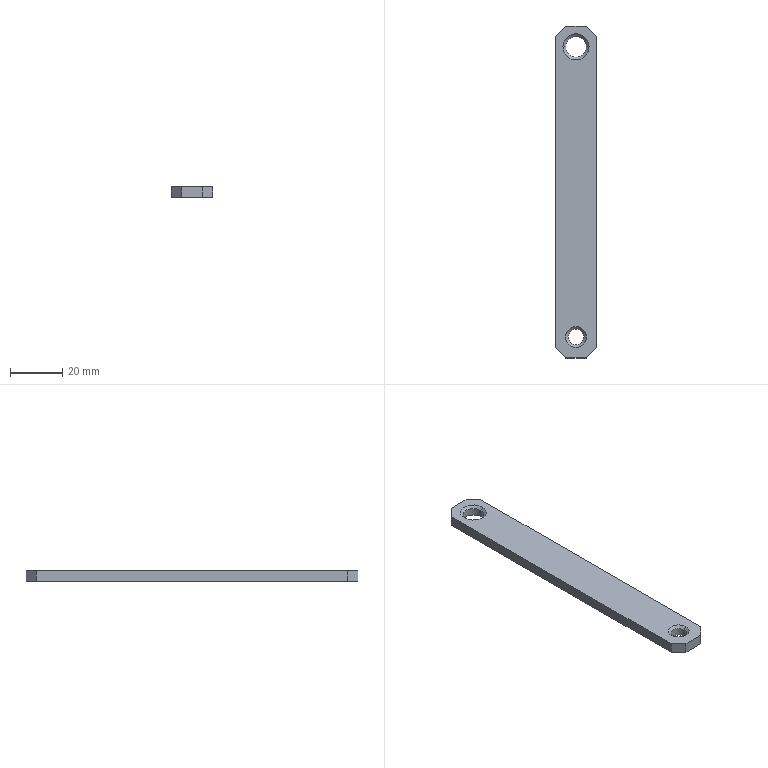Part | STEP file | 8XS174016-2 | 1 solid | 18 faces | box 16 x 127 x 4 mm | volume 7662 mm3 | plane 10 | cone 4 | cylinder 4 | commonest cylinder face diameters 6 x2 8 x2
STEP:
#1=CARTESIAN_POINT('',(0.,0.,0.));
#2=DIRECTION('',(0.,0.,1.));
#3=DIRECTION('',(1.,0.,0.));
#4=AXIS2_PLACEMENT_3D('',#1,#2,#3);
#5=CARTESIAN_POINT('',(4.,119.,3.));
#6=VERTEX_POINT('',#5);
#7=CARTESIAN_POINT('',(5.,119.,4.));
#8=VERTEX_POINT('',#7);
#9=CARTESIAN_POINT('',(4.,119.,3.));
#10=DIRECTION('',(0.7071,0.,0.7071));
#11=VECTOR('',#10,1.);
#12=LINE('',#9,#11);
#13=CARTESIAN_POINT('',(0.,119.,3.));
#14=DIRECTION('',(0.,0.,1.));
#15=DIRECTION('',(1.,0.,0.));
#16=AXIS2_PLACEMENT_3D('',#13,#14,#15);
#17=CONICAL_SURFACE('',#16,4.,0.7854);
#18=CARTESIAN_POINT('',(6.283,0.));
#19=DIRECTION('',(0.,1.));
#20=VECTOR('',#19,1.);
#21=LINE('',#18,#20);
#22=(GEOMETRIC_REPRESENTATION_CONTEXT(2)PARAMETRIC_REPRESENTATION_CONTEXT()REPRESENTATION_CONTEXT('',''));
#23=DEFINITIONAL_REPRESENTATION('',(#21),#22);
#24=PCURVE('',#17,#23);
#25=CARTESIAN_POINT('',(0.,119.,3.));
#26=DIRECTION('',(0.,0.,1.));
#27=DIRECTION('',(1.,0.,0.));
#28=AXIS2_PLACEMENT_3D('',#25,#26,#27);
#29=CONICAL_SURFACE('',#28,4.,0.7854);
#30=CARTESIAN_POINT('',(0.,0.));
#31=DIRECTION('',(0.,1.));
#32=VECTOR('',#31,1.);
#33=LINE('',#30,#32);
#34=(GEOMETRIC_REPRESENTATION_CONTEXT(2)PARAMETRIC_REPRESENTATION_CONTEXT()REPRESENTATION_CONTEXT('',''));
#35=DEFINITIONAL_REPRESENTATION('',(#33),#34);
#36=PCURVE('',#29,#35);
#37=SURFACE_CURVE('',#12,(#24,#36),.PCURVE_S1.);
#38=EDGE_CURVE('',#6,#8,#37,.T.);
#39=ORIENTED_EDGE('',*,*,#38,.T.);
#40=CARTESIAN_POINT('',(-5.,119.,4.));
#41=VERTEX_POINT('',#40);
#42=CARTESIAN_POINT('',(0.,119.,4.));
#43=DIRECTION('',(0.,0.,-1.));
#44=DIRECTION('',(1.,0.,0.));
#45=AXIS2_PLACEMENT_3D('',#42,#43,#44);
#46=CIRCLE('',#45,5.);
#47=CARTESIAN_POINT('',(6.283,1.));
#48=DIRECTION('',(-1.,0.));
#49=VECTOR('',#48,1.);
#50=LINE('',#47,#49);
#51=(GEOMETRIC_REPRESENTATION_CONTEXT(2)PARAMETRIC_REPRESENTATION_CONTEXT()REPRESENTATION_CONTEXT('',''));
#52=DEFINITIONAL_REPRESENTATION('',(#50),#51);
#53=PCURVE('',#17,#52);
#54=CARTESIAN_POINT('',(67.5,63.5,4.));
#55=DIRECTION('',(0.,0.,1.));
#56=DIRECTION('',(1.,0.,0.));
#57=AXIS2_PLACEMENT_3D('',#54,#55,#56);
#58=PLANE('',#57);
#59=CARTESIAN_POINT('',(-62.5,55.5));
#60=CARTESIAN_POINT('',(-62.5,46.84));
#61=CARTESIAN_POINT('',(-70.,51.17));
#62=CARTESIAN_POINT('',(-77.5,55.5));
#63=CARTESIAN_POINT('',(-70.,59.83));
#64=CARTESIAN_POINT('',(-62.5,64.16));
#65=CARTESIAN_POINT('',(-62.5,55.5));
#66=(BOUNDED_CURVE()B_SPLINE_CURVE(2,(#59,#60,#61,#62,#63,#64,#65),.UNSPECIFIED.,.T.,.F.)B_SPLINE_CURVE_WITH_KNOTS((1,2,2,2,2,1),(-2.094,0.,2.094,4.189,6.283,8.378),.UNSPECIFIED.)CURVE()GEOMETRIC_REPRESENTATION_ITEM()RATIONAL_B_SPLINE_CURVE((1.,0.5,1.,0.5,1.,0.5,1.))REPRESENTATION_ITEM(''));
#67=(GEOMETRIC_REPRESENTATION_CONTEXT(2)PARAMETRIC_REPRESENTATION_CONTEXT()REPRESENTATION_CONTEXT('',''));
#68=DEFINITIONAL_REPRESENTATION('',(#66),#67);
#69=PCURVE('',#58,#68);
#70=SURFACE_CURVE('',#46,(#53,#69),.PCURVE_S1.);
#71=EDGE_CURVE('',#8,#41,#70,.T.);
#72=ORIENTED_EDGE('',*,*,#71,.T.);
#73=CARTESIAN_POINT('',(-4.,119.,3.));
#74=VERTEX_POINT('',#73);
#75=CARTESIAN_POINT('',(-4.,119.,3.));
#76=DIRECTION('',(-0.7071,0.,0.7071));
#77=VECTOR('',#76,1.);
#78=LINE('',#75,#77);
#79=CARTESIAN_POINT('',(3.142,0.));
#80=DIRECTION('',(0.,1.));
#81=VECTOR('',#80,1.);
#82=LINE('',#79,#81);
#83=(GEOMETRIC_REPRESENTATION_CONTEXT(2)PARAMETRIC_REPRESENTATION_CONTEXT()REPRESENTATION_CONTEXT('',''));
#84=DEFINITIONAL_REPRESENTATION('',(#82),#83);
#85=PCURVE('',#17,#84);
#86=CARTESIAN_POINT('',(3.142,0.));
#87=DIRECTION('',(0.,1.));
#88=VECTOR('',#87,1.);
#89=LINE('',#86,#88);
#90=(GEOMETRIC_REPRESENTATION_CONTEXT(2)PARAMETRIC_REPRESENTATION_CONTEXT()REPRESENTATION_CONTEXT('',''));
#91=DEFINITIONAL_REPRESENTATION('',(#89),#90);
#92=PCURVE('',#29,#91);
#93=SURFACE_CURVE('',#78,(#85,#92),.PCURVE_S1.);
#94=EDGE_CURVE('',#74,#41,#93,.T.);
#95=ORIENTED_EDGE('',*,*,#94,.F.);
#96=CARTESIAN_POINT('',(0.,119.,3.));
#97=DIRECTION('',(0.,0.,1.));
#98=DIRECTION('',(1.,0.,0.));
#99=AXIS2_PLACEMENT_3D('',#96,#97,#98);
#100=CIRCLE('',#99,4.);
#101=CARTESIAN_POINT('',(0.,0.));
#102=DIRECTION('',(1.,0.));
#103=VECTOR('',#102,1.);
#104=LINE('',#101,#103);
#105=(GEOMETRIC_REPRESENTATION_CONTEXT(2)PARAMETRIC_REPRESENTATION_CONTEXT()REPRESENTATION_CONTEXT('',''));
#106=DEFINITIONAL_REPRESENTATION('',(#104),#105);
#107=PCURVE('',#17,#106);
#108=CARTESIAN_POINT('',(0.,119.,-6.));
#109=DIRECTION('',(0.,0.,1.));
#110=DIRECTION('',(1.,0.,0.));
#111=AXIS2_PLACEMENT_3D('',#108,#109,#110);
#112=CYLINDRICAL_SURFACE('',#111,4.);
#113=CARTESIAN_POINT('',(0.,9.));
#114=DIRECTION('',(1.,0.));
#115=VECTOR('',#114,1.);
#116=LINE('',#113,#115);
#117=(GEOMETRIC_REPRESENTATION_CONTEXT(2)PARAMETRIC_REPRESENTATION_CONTEXT()REPRESENTATION_CONTEXT('',''));
#118=DEFINITIONAL_REPRESENTATION('',(#116),#117);
#119=PCURVE('',#112,#118);
#120=SURFACE_CURVE('',#100,(#107,#119),.PCURVE_S1.);
#121=EDGE_CURVE('',#74,#6,#120,.T.);
#122=ORIENTED_EDGE('',*,*,#121,.T.);
#123=EDGE_LOOP('',(#39,#72,#95,#122));
#124=FACE_BOUND('',#123,.F.);
#125=ADVANCED_FACE('',(#124),#17,.F.);
#126=CARTESIAN_POINT('',(4.,119.,0.));
#127=VERTEX_POINT('',#126);
#128=CARTESIAN_POINT('',(4.,119.,-6.));
#129=DIRECTION('',(0.,0.,1.));
#130=VECTOR('',#129,1.);
#131=LINE('',#128,#130);
#132=CARTESIAN_POINT('',(6.283,0.));
#133=DIRECTION('',(0.,1.));
#134=VECTOR('',#133,1.);
#135=LINE('',#132,#134);
#136=(GEOMETRIC_REPRESENTATION_CONTEXT(2)PARAMETRIC_REPRESENTATION_CONTEXT()REPRESENTATION_CONTEXT('',''));
#137=DEFINITIONAL_REPRESENTATION('',(#135),#136);
#138=PCURVE('',#112,#137);
#139=CARTESIAN_POINT('',(0.,119.,-6.));
#140=DIRECTION('',(0.,0.,1.));
#141=DIRECTION('',(1.,0.,0.));
#142=AXIS2_PLACEMENT_3D('',#139,#140,#141);
#143=CYLINDRICAL_SURFACE('',#142,4.);
#144=CARTESIAN_POINT('',(0.,0.));
#145=DIRECTION('',(0.,1.));
#146=VECTOR('',#145,1.);
#147=LINE('',#144,#146);
#148=(GEOMETRIC_REPRESENTATION_CONTEXT(2)PARAMETRIC_REPRESENTATION_CONTEXT()REPRESENTATION_CONTEXT('',''));
#149=DEFINITIONAL_REPRESENTATION('',(#147),#148);
#150=PCURVE('',#143,#149);
#151=SURFACE_CURVE('',#131,(#138,#150),.PCURVE_S1.);
#152=EDGE_CURVE('',#127,#6,#151,.T.);
#153=ORIENTED_EDGE('',*,*,#152,.T.);
#154=ORIENTED_EDGE('',*,*,#121,.F.);
#155=CARTESIAN_POINT('',(-4.,119.,0.));
#156=VERTEX_POINT('',#155);
#157=CARTESIAN_POINT('',(-4.,119.,-6.));
#158=DIRECTION('',(0.,0.,1.));
#159=VECTOR('',#158,1.);
#160=LINE('',#157,#159);
#161=CARTESIAN_POINT('',(3.142,0.));
#162=DIRECTION('',(0.,1.));
#163=VECTOR('',#162,1.);
#164=LINE('',#161,#163);
#165=(GEOMETRIC_REPRESENTATION_CONTEXT(2)PARAMETRIC_REPRESENTATION_CONTEXT()REPRESENTATION_CONTEXT('',''));
#166=DEFINITIONAL_REPRESENTATION('',(#164),#165);
#167=PCURVE('',#112,#166);
#168=CARTESIAN_POINT('',(3.142,0.));
#169=DIRECTION('',(0.,1.));
#170=VECTOR('',#169,1.);
#171=LINE('',#168,#170);
#172=(GEOMETRIC_REPRESENTATION_CONTEXT(2)PARAMETRIC_REPRESENTATION_CONTEXT()REPRESENTATION_CONTEXT('',''));
#173=DEFINITIONAL_REPRESENTATION('',(#171),#172);
#174=PCURVE('',#143,#173);
#175=SURFACE_CURVE('',#160,(#167,#174),.PCURVE_S1.);
#176=EDGE_CURVE('',#156,#74,#175,.T.);
#177=ORIENTED_EDGE('',*,*,#176,.F.);
#178=CARTESIAN_POINT('',(0.,119.,0.));
#179=DIRECTION('',(0.,0.,1.));
#180=DIRECTION('',(1.,0.,0.));
#181=AXIS2_PLACEMENT_3D('',#178,#179,#180);
#182=CIRCLE('',#181,4.);
#183=CARTESIAN_POINT('',(0.,6.));
#184=DIRECTION('',(1.,0.));
#185=VECTOR('',#184,1.);
#186=LINE('',#183,#185);
#187=(GEOMETRIC_REPRESENTATION_CONTEXT(2)PARAMETRIC_REPRESENTATION_CONTEXT()REPRESENTATION_CONTEXT('',''));
#188=DEFINITIONAL_REPRESENTATION('',(#186),#187);
#189=PCURVE('',#112,#188);
#190=CARTESIAN_POINT('',(67.5,63.5,0.));
#191=DIRECTION('',(0.,0.,1.));
#192=DIRECTION('',(1.,0.,0.));
#193=AXIS2_PLACEMENT_3D('',#190,#191,#192);
#194=PLANE('',#193);
#195=CARTESIAN_POINT('',(-67.5,55.5));
#196=DIRECTION('',(1.,0.));
#197=AXIS2_PLACEMENT_2D('',#195,#196);
#198=CIRCLE('',#197,4.);
#199=(GEOMETRIC_REPRESENTATION_CONTEXT(2)PARAMETRIC_REPRESENTATION_CONTEXT()REPRESENTATION_CONTEXT('',''));
#200=DEFINITIONAL_REPRESENTATION('',(#198),#199);
#201=PCURVE('',#194,#200);
#202=SURFACE_CURVE('',#182,(#189,#201),.PCURVE_S1.);
#203=EDGE_CURVE('',#156,#127,#202,.T.);
#204=ORIENTED_EDGE('',*,*,#203,.T.);
#205=EDGE_LOOP('',(#153,#154,#177,#204));
#206=FACE_BOUND('',#205,.F.);
#207=ADVANCED_FACE('',(#206),#112,.F.);
#208=CARTESIAN_POINT('',(3.,8.,3.));
#209=VERTEX_POINT('',#208);
#210=CARTESIAN_POINT('',(4.,8.,4.));
#211=VERTEX_POINT('',#210);
#212=CARTESIAN_POINT('',(4.,8.,4.));
#213=DIRECTION('',(0.7071,0.,0.7071));
#214=VECTOR('',#213,1.);
#215=LINE('',#212,#214);
#216=CARTESIAN_POINT('',(0.,8.,4.));
#217=DIRECTION('',(0.,0.,1.));
#218=DIRECTION('',(1.,0.,0.));
#219=AXIS2_PLACEMENT_3D('',#216,#217,#218);
#220=CONICAL_SURFACE('',#219,4.,0.7854);
#221=CARTESIAN_POINT('',(6.283,0.));
#222=DIRECTION('',(0.,1.));
#223=VECTOR('',#222,1.);
#224=LINE('',#221,#223);
#225=(GEOMETRIC_REPRESENTATION_CONTEXT(2)PARAMETRIC_REPRESENTATION_CONTEXT()REPRESENTATION_CONTEXT('',''));
#226=DEFINITIONAL_REPRESENTATION('',(#224),#225);
#227=PCURVE('',#220,#226);
#228=CARTESIAN_POINT('',(0.,8.,4.));
#229=DIRECTION('',(0.,0.,1.));
#230=DIRECTION('',(1.,0.,0.));
#231=AXIS2_PLACEMENT_3D('',#228,#229,#230);
#232=CONICAL_SURFACE('',#231,4.,0.7854);
#233=CARTESIAN_POINT('',(0.,0.));
#234=DIRECTION('',(0.,1.));
#235=VECTOR('',#234,1.);
#236=LINE('',#233,#235);
#237=(GEOMETRIC_REPRESENTATION_CONTEXT(2)PARAMETRIC_REPRESENTATION_CONTEXT()REPRESENTATION_CONTEXT('',''));
#238=DEFINITIONAL_REPRESENTATION('',(#236),#237);
#239=PCURVE('',#232,#238);
#240=SURFACE_CURVE('',#215,(#227,#239),.PCURVE_S1.);
#241=EDGE_CURVE('',#209,#211,#240,.T.);
#242=ORIENTED_EDGE('',*,*,#241,.T.);
#243=CARTESIAN_POINT('',(-4.,8.,4.));
#244=VERTEX_POINT('',#243);
#245=CARTESIAN_POINT('',(0.,8.,4.));
#246=DIRECTION('',(0.,0.,1.));
#247=DIRECTION('',(1.,0.,0.));
#248=AXIS2_PLACEMENT_3D('',#245,#246,#247);
#249=CIRCLE('',#248,4.);
#250=CARTESIAN_POINT('',(0.,0.));
#251=DIRECTION('',(1.,0.));
#252=VECTOR('',#251,1.);
#253=LINE('',#250,#252);
#254=(GEOMETRIC_REPRESENTATION_CONTEXT(2)PARAMETRIC_REPRESENTATION_CONTEXT()REPRESENTATION_CONTEXT('',''));
#255=DEFINITIONAL_REPRESENTATION('',(#253),#254);
#256=PCURVE('',#220,#255);
#257=CARTESIAN_POINT('',(-67.5,-55.5));
#258=DIRECTION('',(1.,0.));
#259=AXIS2_PLACEMENT_2D('',#257,#258);
#260=CIRCLE('',#259,4.);
#261=(GEOMETRIC_REPRESENTATION_CONTEXT(2)PARAMETRIC_REPRESENTATION_CONTEXT()REPRESENTATION_CONTEXT('',''));
#262=DEFINITIONAL_REPRESENTATION('',(#260),#261);
#263=PCURVE('',#58,#262);
#264=SURFACE_CURVE('',#249,(#256,#263),.PCURVE_S1.);
#265=EDGE_CURVE('',#244,#211,#264,.T.);
#266=ORIENTED_EDGE('',*,*,#265,.F.);
#267=CARTESIAN_POINT('',(-3.,8.,3.));
#268=VERTEX_POINT('',#267);
#269=CARTESIAN_POINT('',(-4.,8.,4.));
#270=DIRECTION('',(-0.7071,0.,0.7071));
#271=VECTOR('',#270,1.);
#272=LINE('',#269,#271);
#273=CARTESIAN_POINT('',(3.142,0.));
#274=DIRECTION('',(0.,1.));
#275=VECTOR('',#274,1.);
#276=LINE('',#273,#275);
#277=(GEOMETRIC_REPRESENTATION_CONTEXT(2)PARAMETRIC_REPRESENTATION_CONTEXT()REPRESENTATION_CONTEXT('',''));
#278=DEFINITIONAL_REPRESENTATION('',(#276),#277);
#279=PCURVE('',#220,#278);
#280=CARTESIAN_POINT('',(3.142,0.));
#281=DIRECTION('',(0.,1.));
#282=VECTOR('',#281,1.);
#283=LINE('',#280,#282);
#284=(GEOMETRIC_REPRESENTATION_CONTEXT(2)PARAMETRIC_REPRESENTATION_CONTEXT()REPRESENTATION_CONTEXT('',''));
#285=DEFINITIONAL_REPRESENTATION('',(#283),#284);
#286=PCURVE('',#232,#285);
#287=SURFACE_CURVE('',#272,(#279,#286),.PCURVE_S1.);
#288=EDGE_CURVE('',#268,#244,#287,.T.);
#289=ORIENTED_EDGE('',*,*,#288,.F.);
#290=CARTESIAN_POINT('',(0.,8.,3.));
#291=DIRECTION('',(0.,0.,1.));
#292=DIRECTION('',(1.,0.,0.));
#293=AXIS2_PLACEMENT_3D('',#290,#291,#292);
#294=CIRCLE('',#293,3.);
#295=CARTESIAN_POINT('',(0.,-1.));
#296=DIRECTION('',(1.,0.));
#297=VECTOR('',#296,1.);
#298=LINE('',#295,#297);
#299=(GEOMETRIC_REPRESENTATION_CONTEXT(2)PARAMETRIC_REPRESENTATION_CONTEXT()REPRESENTATION_CONTEXT('',''));
#300=DEFINITIONAL_REPRESENTATION('',(#298),#299);
#301=PCURVE('',#220,#300);
#302=CARTESIAN_POINT('',(0.,8.,4.));
#303=DIRECTION('',(0.,0.,1.));
#304=DIRECTION('',(1.,0.,0.));
#305=AXIS2_PLACEMENT_3D('',#302,#303,#304);
#306=CYLINDRICAL_SURFACE('',#305,3.);
#307=CARTESIAN_POINT('',(0.,-1.));
#308=DIRECTION('',(1.,0.));
#309=VECTOR('',#308,1.);
#310=LINE('',#307,#309);
#311=(GEOMETRIC_REPRESENTATION_CONTEXT(2)PARAMETRIC_REPRESENTATION_CONTEXT()REPRESENTATION_CONTEXT('',''));
#312=DEFINITIONAL_REPRESENTATION('',(#310),#311);
#313=PCURVE('',#306,#312);
#314=SURFACE_CURVE('',#294,(#301,#313),.PCURVE_S1.);
#315=EDGE_CURVE('',#268,#209,#314,.T.);
#316=ORIENTED_EDGE('',*,*,#315,.T.);
#317=EDGE_LOOP('',(#242,#266,#289,#316));
#318=FACE_BOUND('',#317,.F.);
#319=ADVANCED_FACE('',(#318),#220,.F.);
#320=CARTESIAN_POINT('',(3.,8.,0.));
#321=VERTEX_POINT('',#320);
#322=CARTESIAN_POINT('',(3.,8.,4.));
#323=DIRECTION('',(0.,0.,1.));
#324=VECTOR('',#323,1.);
#325=LINE('',#322,#324);
#326=CARTESIAN_POINT('',(6.283,0.));
#327=DIRECTION('',(0.,1.));
#328=VECTOR('',#327,1.);
#329=LINE('',#326,#328);
#330=(GEOMETRIC_REPRESENTATION_CONTEXT(2)PARAMETRIC_REPRESENTATION_CONTEXT()REPRESENTATION_CONTEXT('',''));
#331=DEFINITIONAL_REPRESENTATION('',(#329),#330);
#332=PCURVE('',#306,#331);
#333=CARTESIAN_POINT('',(0.,8.,4.));
#334=DIRECTION('',(0.,0.,1.));
#335=DIRECTION('',(1.,0.,0.));
#336=AXIS2_PLACEMENT_3D('',#333,#334,#335);
#337=CYLINDRICAL_SURFACE('',#336,3.);
#338=CARTESIAN_POINT('',(0.,0.));
#339=DIRECTION('',(0.,1.));
#340=VECTOR('',#339,1.);
#341=LINE('',#338,#340);
#342=(GEOMETRIC_REPRESENTATION_CONTEXT(2)PARAMETRIC_REPRESENTATION_CONTEXT()REPRESENTATION_CONTEXT('',''));
#343=DEFINITIONAL_REPRESENTATION('',(#341),#342);
#344=PCURVE('',#337,#343);
#345=SURFACE_CURVE('',#325,(#332,#344),.PCURVE_S1.);
#346=EDGE_CURVE('',#321,#209,#345,.T.);
#347=ORIENTED_EDGE('',*,*,#346,.T.);
#348=ORIENTED_EDGE('',*,*,#315,.F.);
#349=CARTESIAN_POINT('',(-3.,8.,0.));
#350=VERTEX_POINT('',#349);
#351=CARTESIAN_POINT('',(-3.,8.,4.));
#352=DIRECTION('',(0.,0.,1.));
#353=VECTOR('',#352,1.);
#354=LINE('',#351,#353);
#355=CARTESIAN_POINT('',(3.142,0.));
#356=DIRECTION('',(0.,1.));
#357=VECTOR('',#356,1.);
#358=LINE('',#355,#357);
#359=(GEOMETRIC_REPRESENTATION_CONTEXT(2)PARAMETRIC_REPRESENTATION_CONTEXT()REPRESENTATION_CONTEXT('',''));
#360=DEFINITIONAL_REPRESENTATION('',(#358),#359);
#361=PCURVE('',#306,#360);
#362=CARTESIAN_POINT('',(3.142,0.));
#363=DIRECTION('',(0.,1.));
#364=VECTOR('',#363,1.);
#365=LINE('',#362,#364);
#366=(GEOMETRIC_REPRESENTATION_CONTEXT(2)PARAMETRIC_REPRESENTATION_CONTEXT()REPRESENTATION_CONTEXT('',''));
#367=DEFINITIONAL_REPRESENTATION('',(#365),#366);
#368=PCURVE('',#337,#367);
#369=SURFACE_CURVE('',#354,(#361,#368),.PCURVE_S1.);
#370=EDGE_CURVE('',#350,#268,#369,.T.);
#371=ORIENTED_EDGE('',*,*,#370,.F.);
#372=CARTESIAN_POINT('',(0.,8.,0.));
#373=DIRECTION('',(0.,0.,1.));
#374=DIRECTION('',(1.,0.,0.));
#375=AXIS2_PLACEMENT_3D('',#372,#373,#374);
#376=CIRCLE('',#375,3.);
#377=CARTESIAN_POINT('',(0.,-4.));
#378=DIRECTION('',(1.,0.));
#379=VECTOR('',#378,1.);
#380=LINE('',#377,#379);
#381=(GEOMETRIC_REPRESENTATION_CONTEXT(2)PARAMETRIC_REPRESENTATION_CONTEXT()REPRESENTATION_CONTEXT('',''));
#382=DEFINITIONAL_REPRESENTATION('',(#380),#381);
#383=PCURVE('',#306,#382);
#384=CARTESIAN_POINT('',(-67.5,-55.5));
#385=DIRECTION('',(1.,0.));
#386=AXIS2_PLACEMENT_2D('',#384,#385);
#387=CIRCLE('',#386,3.);
#388=(GEOMETRIC_REPRESENTATION_CONTEXT(2)PARAMETRIC_REPRESENTATION_CONTEXT()REPRESENTATION_CONTEXT('',''));
#389=DEFINITIONAL_REPRESENTATION('',(#387),#388);
#390=PCURVE('',#194,#389);
#391=SURFACE_CURVE('',#376,(#383,#390),.PCURVE_S1.);
#392=EDGE_CURVE('',#350,#321,#391,.T.);
#393=ORIENTED_EDGE('',*,*,#392,.T.);
#394=EDGE_LOOP('',(#347,#348,#371,#393));
#395=FACE_BOUND('',#394,.F.);
#396=ADVANCED_FACE('',(#395),#306,.F.);
#397=CARTESIAN_POINT('',(4.,0.,4.));
#398=VERTEX_POINT('',#397);
#399=CARTESIAN_POINT('',(8.,4.,4.));
#400=VERTEX_POINT('',#399);
#401=CARTESIAN_POINT('',(4.,0.,4.));
#402=DIRECTION('',(0.7071,0.7071,0.));
#403=VECTOR('',#402,1.);
#404=LINE('',#401,#403);
#405=CARTESIAN_POINT('',(4.,0.,0.));
#406=DIRECTION('',(0.7071,-0.7071,0.));
#407=DIRECTION('',(0.7071,0.7071,0.));
#408=AXIS2_PLACEMENT_3D('',#405,#406,#407);
#409=PLANE('',#408);
#410=CARTESIAN_POINT('',(0.,4.));
#411=DIRECTION('',(1.,0.));
#412=VECTOR('',#411,1.);
#413=LINE('',#410,#412);
#414=(GEOMETRIC_REPRESENTATION_CONTEXT(2)PARAMETRIC_REPRESENTATION_CONTEXT()REPRESENTATION_CONTEXT('',''));
#415=DEFINITIONAL_REPRESENTATION('',(#413),#414);
#416=PCURVE('',#409,#415);
#417=CARTESIAN_POINT('',(-63.5,-63.5));
#418=DIRECTION('',(0.7071,0.7071));
#419=VECTOR('',#418,1.);
#420=LINE('',#417,#419);
#421=(GEOMETRIC_REPRESENTATION_CONTEXT(2)PARAMETRIC_REPRESENTATION_CONTEXT()REPRESENTATION_CONTEXT('',''));
#422=DEFINITIONAL_REPRESENTATION('',(#420),#421);
#423=PCURVE('',#58,#422);
#424=SURFACE_CURVE('',#404,(#416,#423),.PCURVE_S1.);
#425=EDGE_CURVE('',#398,#400,#424,.T.);
#426=ORIENTED_EDGE('',*,*,#425,.F.);
#427=CARTESIAN_POINT('',(4.,0.,0.));
#428=VERTEX_POINT('',#427);
#429=CARTESIAN_POINT('',(4.,0.,0.));
#430=DIRECTION('',(0.,0.,1.));
#431=VECTOR('',#430,1.);
#432=LINE('',#429,#431);
#433=CARTESIAN_POINT('',(0.,0.));
#434=DIRECTION('',(0.,1.));
#435=VECTOR('',#434,1.);
#436=LINE('',#433,#435);
#437=(GEOMETRIC_REPRESENTATION_CONTEXT(2)PARAMETRIC_REPRESENTATION_CONTEXT()REPRESENTATION_CONTEXT('',''));
#438=DEFINITIONAL_REPRESENTATION('',(#436),#437);
#439=PCURVE('',#409,#438);
#440=CARTESIAN_POINT('',(-4.,0.,0.));
#441=DIRECTION('',(0.,-1.,0.));
#442=DIRECTION('',(1.,0.,0.));
#443=AXIS2_PLACEMENT_3D('',#440,#441,#442);
#444=PLANE('',#443);
#445=CARTESIAN_POINT('',(8.,0.));
#446=DIRECTION('',(0.,1.));
#447=VECTOR('',#446,1.);
#448=LINE('',#445,#447);
#449=(GEOMETRIC_REPRESENTATION_CONTEXT(2)PARAMETRIC_REPRESENTATION_CONTEXT()REPRESENTATION_CONTEXT('',''));
#450=DEFINITIONAL_REPRESENTATION('',(#448),#449);
#451=PCURVE('',#444,#450);
#452=SURFACE_CURVE('',#432,(#439,#451),.PCURVE_S1.);
#453=EDGE_CURVE('',#428,#398,#452,.T.);
#454=ORIENTED_EDGE('',*,*,#453,.F.);
#455=CARTESIAN_POINT('',(8.,4.,0.));
#456=VERTEX_POINT('',#455);
#457=CARTESIAN_POINT('',(4.,0.,0.));
#458=DIRECTION('',(0.7071,0.7071,0.));
#459=VECTOR('',#458,1.);
#460=LINE('',#457,#459);
#461=CARTESIAN_POINT('',(0.,0.));
#462=DIRECTION('',(1.,0.));
#463=VECTOR('',#462,1.);
#464=LINE('',#461,#463);
#465=(GEOMETRIC_REPRESENTATION_CONTEXT(2)PARAMETRIC_REPRESENTATION_CONTEXT()REPRESENTATION_CONTEXT('',''));
#466=DEFINITIONAL_REPRESENTATION('',(#464),#465);
#467=PCURVE('',#409,#466);
#468=CARTESIAN_POINT('',(-63.5,-63.5));
#469=DIRECTION('',(0.7071,0.7071));
#470=VECTOR('',#469,1.);
#471=LINE('',#468,#470);
#472=(GEOMETRIC_REPRESENTATION_CONTEXT(2)PARAMETRIC_REPRESENTATION_CONTEXT()REPRESENTATION_CONTEXT('',''));
#473=DEFINITIONAL_REPRESENTATION('',(#471),#472);
#474=PCURVE('',#194,#473);
#475=SURFACE_CURVE('',#460,(#467,#474),.PCURVE_S1.);
#476=EDGE_CURVE('',#428,#456,#475,.T.);
#477=ORIENTED_EDGE('',*,*,#476,.T.);
#478=CARTESIAN_POINT('',(8.,4.,0.));
#479=DIRECTION('',(0.,0.,1.));
#480=VECTOR('',#479,1.);
#481=LINE('',#478,#480);
#482=CARTESIAN_POINT('',(5.657,0.));
#483=DIRECTION('',(0.,1.));
#484=VECTOR('',#483,1.);
#485=LINE('',#482,#484);
#486=(GEOMETRIC_REPRESENTATION_CONTEXT(2)PARAMETRIC_REPRESENTATION_CONTEXT()REPRESENTATION_CONTEXT('',''));
#487=DEFINITIONAL_REPRESENTATION('',(#485),#486);
#488=PCURVE('',#409,#487);
#489=CARTESIAN_POINT('',(8.,4.,0.));
#490=DIRECTION('',(1.,0.,0.));
#491=DIRECTION('',(0.,1.,0.));
#492=AXIS2_PLACEMENT_3D('',#489,#490,#491);
#493=PLANE('',#492);
#494=CARTESIAN_POINT('',(0.,0.));
#495=DIRECTION('',(0.,1.));
#496=VECTOR('',#495,1.);
#497=LINE('',#494,#496);
#498=(GEOMETRIC_REPRESENTATION_CONTEXT(2)PARAMETRIC_REPRESENTATION_CONTEXT()REPRESENTATION_CONTEXT('',''));
#499=DEFINITIONAL_REPRESENTATION('',(#497),#498);
#500=PCURVE('',#493,#499);
#501=SURFACE_CURVE('',#481,(#488,#500),.PCURVE_S1.);
#502=EDGE_CURVE('',#456,#400,#501,.T.);
#503=ORIENTED_EDGE('',*,*,#502,.T.);
#504=EDGE_LOOP('',(#426,#454,#477,#503));
#505=FACE_BOUND('',#504,.T.);
#506=ADVANCED_FACE('',(#505),#409,.T.);
#507=CARTESIAN_POINT('',(-4.,0.,4.));
#508=VERTEX_POINT('',#507);
#509=CARTESIAN_POINT('',(-4.,0.,4.));
#510=DIRECTION('',(1.,0.,0.));
#511=VECTOR('',#510,1.);
#512=LINE('',#509,#511);
#513=CARTESIAN_POINT('',(0.,4.));
#514=DIRECTION('',(1.,0.));
#515=VECTOR('',#514,1.);
#516=LINE('',#513,#515);
#517=(GEOMETRIC_REPRESENTATION_CONTEXT(2)PARAMETRIC_REPRESENTATION_CONTEXT()REPRESENTATION_CONTEXT('',''));
#518=DEFINITIONAL_REPRESENTATION('',(#516),#517);
#519=PCURVE('',#444,#518);
#520=CARTESIAN_POINT('',(-71.5,-63.5));
#521=DIRECTION('',(1.,0.));
#522=VECTOR('',#521,1.);
#523=LINE('',#520,#522);
#524=(GEOMETRIC_REPRESENTATION_CONTEXT(2)PARAMETRIC_REPRESENTATION_CONTEXT()REPRESENTATION_CONTEXT('',''));
#525=DEFINITIONAL_REPRESENTATION('',(#523),#524);
#526=PCURVE('',#58,#525);
#527=SURFACE_CURVE('',#512,(#519,#526),.PCURVE_S1.);
#528=EDGE_CURVE('',#508,#398,#527,.T.);
#529=ORIENTED_EDGE('',*,*,#528,.F.);
#530=CARTESIAN_POINT('',(-4.,0.,0.));
#531=VERTEX_POINT('',#530);
#532=CARTESIAN_POINT('',(-4.,0.,0.));
#533=DIRECTION('',(0.,0.,1.));
#534=VECTOR('',#533,1.);
#535=LINE('',#532,#534);
#536=CARTESIAN_POINT('',(0.,0.));
#537=DIRECTION('',(0.,1.));
#538=VECTOR('',#537,1.);
#539=LINE('',#536,#538);
#540=(GEOMETRIC_REPRESENTATION_CONTEXT(2)PARAMETRIC_REPRESENTATION_CONTEXT()REPRESENTATION_CONTEXT('',''));
#541=DEFINITIONAL_REPRESENTATION('',(#539),#540);
#542=PCURVE('',#444,#541);
#543=CARTESIAN_POINT('',(-8.,4.,0.));
#544=DIRECTION('',(-0.7071,-0.7071,0.));
#545=DIRECTION('',(0.7071,-0.7071,0.));
#546=AXIS2_PLACEMENT_3D('',#543,#544,#545);
#547=PLANE('',#546);
#548=CARTESIAN_POINT('',(5.657,0.));
#549=DIRECTION('',(0.,1.));
#550=VECTOR('',#549,1.);
#551=LINE('',#548,#550);
#552=(GEOMETRIC_REPRESENTATION_CONTEXT(2)PARAMETRIC_REPRESENTATION_CONTEXT()REPRESENTATION_CONTEXT('',''));
#553=DEFINITIONAL_REPRESENTATION('',(#551),#552);
#554=PCURVE('',#547,#553);
#555=SURFACE_CURVE('',#535,(#542,#554),.PCURVE_S1.);
#556=EDGE_CURVE('',#531,#508,#555,.T.);
#557=ORIENTED_EDGE('',*,*,#556,.F.);
#558=CARTESIAN_POINT('',(-4.,0.,0.));
#559=DIRECTION('',(1.,0.,0.));
#560=VECTOR('',#559,1.);
#561=LINE('',#558,#560);
#562=CARTESIAN_POINT('',(0.,0.));
#563=DIRECTION('',(1.,0.));
#564=VECTOR('',#563,1.);
#565=LINE('',#562,#564);
#566=(GEOMETRIC_REPRESENTATION_CONTEXT(2)PARAMETRIC_REPRESENTATION_CONTEXT()REPRESENTATION_CONTEXT('',''));
#567=DEFINITIONAL_REPRESENTATION('',(#565),#566);
#568=PCURVE('',#444,#567);
#569=CARTESIAN_POINT('',(-71.5,-63.5));
#570=DIRECTION('',(1.,0.));
#571=VECTOR('',#570,1.);
#572=LINE('',#569,#571);
#573=(GEOMETRIC_REPRESENTATION_CONTEXT(2)PARAMETRIC_REPRESENTATION_CONTEXT()REPRESENTATION_CONTEXT('',''));
#574=DEFINITIONAL_REPRESENTATION('',(#572),#573);
#575=PCURVE('',#194,#574);
#576=SURFACE_CURVE('',#561,(#568,#575),.PCURVE_S1.);
#577=EDGE_CURVE('',#531,#428,#576,.T.);
#578=ORIENTED_EDGE('',*,*,#577,.T.);
#579=ORIENTED_EDGE('',*,*,#453,.T.);
#580=EDGE_LOOP('',(#529,#557,#578,#579));
#581=FACE_BOUND('',#580,.T.);
#582=ADVANCED_FACE('',(#581),#444,.T.);
#583=CARTESIAN_POINT('',(-8.,4.,4.));
#584=VERTEX_POINT('',#583);
#585=CARTESIAN_POINT('',(-8.,4.,4.));
#586=DIRECTION('',(0.7071,-0.7071,0.));
#587=VECTOR('',#586,1.);
#588=LINE('',#585,#587);
#589=CARTESIAN_POINT('',(0.,4.));
#590=DIRECTION('',(1.,0.));
#591=VECTOR('',#590,1.);
#592=LINE('',#589,#591);
#593=(GEOMETRIC_REPRESENTATION_CONTEXT(2)PARAMETRIC_REPRESENTATION_CONTEXT()REPRESENTATION_CONTEXT('',''));
#594=DEFINITIONAL_REPRESENTATION('',(#592),#593);
#595=PCURVE('',#547,#594);
#596=CARTESIAN_POINT('',(-75.5,-59.5));
#597=DIRECTION('',(0.7071,-0.7071));
#598=VECTOR('',#597,1.);
#599=LINE('',#596,#598);
#600=(GEOMETRIC_REPRESENTATION_CONTEXT(2)PARAMETRIC_REPRESENTATION_CONTEXT()REPRESENTATION_CONTEXT('',''));
#601=DEFINITIONAL_REPRESENTATION('',(#599),#600);
#602=PCURVE('',#58,#601);
#603=SURFACE_CURVE('',#588,(#595,#602),.PCURVE_S1.);
#604=EDGE_CURVE('',#584,#508,#603,.T.);
#605=ORIENTED_EDGE('',*,*,#604,.F.);
#606=CARTESIAN_POINT('',(-8.,4.,0.));
#607=VERTEX_POINT('',#606);
#608=CARTESIAN_POINT('',(-8.,4.,0.));
#609=DIRECTION('',(0.,0.,1.));
#610=VECTOR('',#609,1.);
#611=LINE('',#608,#610);
#612=CARTESIAN_POINT('',(0.,0.));
#613=DIRECTION('',(0.,1.));
#614=VECTOR('',#613,1.);
#615=LINE('',#612,#614);
#616=(GEOMETRIC_REPRESENTATION_CONTEXT(2)PARAMETRIC_REPRESENTATION_CONTEXT()REPRESENTATION_CONTEXT('',''));
#617=DEFINITIONAL_REPRESENTATION('',(#615),#616);
#618=PCURVE('',#547,#617);
#619=CARTESIAN_POINT('',(-8.,123.,0.));
#620=DIRECTION('',(-1.,0.,0.));
#621=DIRECTION('',(0.,-1.,0.));
#622=AXIS2_PLACEMENT_3D('',#619,#620,#621);
#623=PLANE('',#622);
#624=CARTESIAN_POINT('',(119.,0.));
#625=DIRECTION('',(0.,1.));
#626=VECTOR('',#625,1.);
#627=LINE('',#624,#626);
#628=(GEOMETRIC_REPRESENTATION_CONTEXT(2)PARAMETRIC_REPRESENTATION_CONTEXT()REPRESENTATION_CONTEXT('',''));
#629=DEFINITIONAL_REPRESENTATION('',(#627),#628);
#630=PCURVE('',#623,#629);
#631=SURFACE_CURVE('',#611,(#618,#630),.PCURVE_S1.);
#632=EDGE_CURVE('',#607,#584,#631,.T.);
#633=ORIENTED_EDGE('',*,*,#632,.F.);
#634=CARTESIAN_POINT('',(-8.,4.,0.));
#635=DIRECTION('',(0.7071,-0.7071,0.));
#636=VECTOR('',#635,1.);
#637=LINE('',#634,#636);
#638=CARTESIAN_POINT('',(0.,0.));
#639=DIRECTION('',(1.,0.));
#640=VECTOR('',#639,1.);
#641=LINE('',#638,#640);
#642=(GEOMETRIC_REPRESENTATION_CONTEXT(2)PARAMETRIC_REPRESENTATION_CONTEXT()REPRESENTATION_CONTEXT('',''));
#643=DEFINITIONAL_REPRESENTATION('',(#641),#642);
#644=PCURVE('',#547,#643);
#645=CARTESIAN_POINT('',(-75.5,-59.5));
#646=DIRECTION('',(0.7071,-0.7071));
#647=VECTOR('',#646,1.);
#648=LINE('',#645,#647);
#649=(GEOMETRIC_REPRESENTATION_CONTEXT(2)PARAMETRIC_REPRESENTATION_CONTEXT()REPRESENTATION_CONTEXT('',''));
#650=DEFINITIONAL_REPRESENTATION('',(#648),#649);
#651=PCURVE('',#194,#650);
#652=SURFACE_CURVE('',#637,(#644,#651),.PCURVE_S1.);
#653=EDGE_CURVE('',#607,#531,#652,.T.);
#654=ORIENTED_EDGE('',*,*,#653,.T.);
#655=ORIENTED_EDGE('',*,*,#556,.T.);
#656=EDGE_LOOP('',(#605,#633,#654,#655));
#657=FACE_BOUND('',#656,.T.);
#658=ADVANCED_FACE('',(#657),#547,.T.);
#659=CARTESIAN_POINT('',(-8.,123.,4.));
#660=VERTEX_POINT('',#659);
#661=CARTESIAN_POINT('',(-8.,123.,4.));
#662=DIRECTION('',(0.,-1.,0.));
#663=VECTOR('',#662,1.);
#664=LINE('',#661,#663);
#665=CARTESIAN_POINT('',(0.,4.));
#666=DIRECTION('',(1.,0.));
#667=VECTOR('',#666,1.);
#668=LINE('',#665,#667);
#669=(GEOMETRIC_REPRESENTATION_CONTEXT(2)PARAMETRIC_REPRESENTATION_CONTEXT()REPRESENTATION_CONTEXT('',''));
#670=DEFINITIONAL_REPRESENTATION('',(#668),#669);
#671=PCURVE('',#623,#670);
#672=CARTESIAN_POINT('',(-75.5,59.5));
#673=DIRECTION('',(0.,-1.));
#674=VECTOR('',#673,1.);
#675=LINE('',#672,#674);
#676=(GEOMETRIC_REPRESENTATION_CONTEXT(2)PARAMETRIC_REPRESENTATION_CONTEXT()REPRESENTATION_CONTEXT('',''));
#677=DEFINITIONAL_REPRESENTATION('',(#675),#676);
#678=PCURVE('',#58,#677);
#679=SURFACE_CURVE('',#664,(#671,#678),.PCURVE_S1.);
#680=EDGE_CURVE('',#660,#584,#679,.T.);
#681=ORIENTED_EDGE('',*,*,#680,.F.);
#682=CARTESIAN_POINT('',(-8.,123.,0.));
#683=VERTEX_POINT('',#682);
#684=CARTESIAN_POINT('',(-8.,123.,0.));
#685=DIRECTION('',(0.,0.,1.));
#686=VECTOR('',#685,1.);
#687=LINE('',#684,#686);
#688=CARTESIAN_POINT('',(0.,0.));
#689=DIRECTION('',(0.,1.));
#690=VECTOR('',#689,1.);
#691=LINE('',#688,#690);
#692=(GEOMETRIC_REPRESENTATION_CONTEXT(2)PARAMETRIC_REPRESENTATION_CONTEXT()REPRESENTATION_CONTEXT('',''));
#693=DEFINITIONAL_REPRESENTATION('',(#691),#692);
#694=PCURVE('',#623,#693);
#695=CARTESIAN_POINT('',(-4.,127.,0.));
#696=DIRECTION('',(-0.7071,0.7071,0.));
#697=DIRECTION('',(-0.7071,-0.7071,0.));
#698=AXIS2_PLACEMENT_3D('',#695,#696,#697);
#699=PLANE('',#698);
#700=CARTESIAN_POINT('',(5.657,0.));
#701=DIRECTION('',(0.,1.));
#702=VECTOR('',#701,1.);
#703=LINE('',#700,#702);
#704=(GEOMETRIC_REPRESENTATION_CONTEXT(2)PARAMETRIC_REPRESENTATION_CONTEXT()REPRESENTATION_CONTEXT('',''));
#705=DEFINITIONAL_REPRESENTATION('',(#703),#704);
#706=PCURVE('',#699,#705);
#707=SURFACE_CURVE('',#687,(#694,#706),.PCURVE_S1.);
#708=EDGE_CURVE('',#683,#660,#707,.T.);
#709=ORIENTED_EDGE('',*,*,#708,.F.);
#710=CARTESIAN_POINT('',(-8.,123.,0.));
#711=DIRECTION('',(0.,-1.,0.));
#712=VECTOR('',#711,1.);
#713=LINE('',#710,#712);
#714=CARTESIAN_POINT('',(0.,0.));
#715=DIRECTION('',(1.,0.));
#716=VECTOR('',#715,1.);
#717=LINE('',#714,#716);
#718=(GEOMETRIC_REPRESENTATION_CONTEXT(2)PARAMETRIC_REPRESENTATION_CONTEXT()REPRESENTATION_CONTEXT('',''));
#719=DEFINITIONAL_REPRESENTATION('',(#717),#718);
#720=PCURVE('',#623,#719);
#721=CARTESIAN_POINT('',(-75.5,59.5));
#722=DIRECTION('',(0.,-1.));
#723=VECTOR('',#722,1.);
#724=LINE('',#721,#723);
#725=(GEOMETRIC_REPRESENTATION_CONTEXT(2)PARAMETRIC_REPRESENTATION_CONTEXT()REPRESENTATION_CONTEXT('',''));
#726=DEFINITIONAL_REPRESENTATION('',(#724),#725);
#727=PCURVE('',#194,#726);
#728=SURFACE_CURVE('',#713,(#720,#727),.PCURVE_S1.);
#729=EDGE_CURVE('',#683,#607,#728,.T.);
#730=ORIENTED_EDGE('',*,*,#729,.T.);
#731=ORIENTED_EDGE('',*,*,#632,.T.);
#732=EDGE_LOOP('',(#681,#709,#730,#731));
#733=FACE_BOUND('',#732,.T.);
#734=ADVANCED_FACE('',(#733),#623,.T.);
#735=CARTESIAN_POINT('',(-4.,127.,4.));
#736=VERTEX_POINT('',#735);
#737=CARTESIAN_POINT('',(-4.,127.,4.));
#738=DIRECTION('',(-0.7071,-0.7071,0.));
#739=VECTOR('',#738,1.);
#740=LINE('',#737,#739);
#741=CARTESIAN_POINT('',(0.,4.));
#742=DIRECTION('',(1.,0.));
#743=VECTOR('',#742,1.);
#744=LINE('',#741,#743);
#745=(GEOMETRIC_REPRESENTATION_CONTEXT(2)PARAMETRIC_REPRESENTATION_CONTEXT()REPRESENTATION_CONTEXT('',''));
#746=DEFINITIONAL_REPRESENTATION('',(#744),#745);
#747=PCURVE('',#699,#746);
#748=CARTESIAN_POINT('',(-71.5,63.5));
#749=DIRECTION('',(-0.7071,-0.7071));
#750=VECTOR('',#749,1.);
#751=LINE('',#748,#750);
#752=(GEOMETRIC_REPRESENTATION_CONTEXT(2)PARAMETRIC_REPRESENTATION_CONTEXT()REPRESENTATION_CONTEXT('',''));
#753=DEFINITIONAL_REPRESENTATION('',(#751),#752);
#754=PCURVE('',#58,#753);
#755=SURFACE_CURVE('',#740,(#747,#754),.PCURVE_S1.);
#756=EDGE_CURVE('',#736,#660,#755,.T.);
#757=ORIENTED_EDGE('',*,*,#756,.F.);
#758=CARTESIAN_POINT('',(-4.,127.,0.));
#759=VERTEX_POINT('',#758);
#760=CARTESIAN_POINT('',(-4.,127.,0.));
#761=DIRECTION('',(0.,0.,1.));
#762=VECTOR('',#761,1.);
#763=LINE('',#760,#762);
#764=CARTESIAN_POINT('',(0.,0.));
#765=DIRECTION('',(0.,1.));
#766=VECTOR('',#765,1.);
#767=LINE('',#764,#766);
#768=(GEOMETRIC_REPRESENTATION_CONTEXT(2)PARAMETRIC_REPRESENTATION_CONTEXT()REPRESENTATION_CONTEXT('',''));
#769=DEFINITIONAL_REPRESENTATION('',(#767),#768);
#770=PCURVE('',#699,#769);
#771=CARTESIAN_POINT('',(4.,127.,0.));
#772=DIRECTION('',(0.,1.,0.));
#773=DIRECTION('',(0.,0.,1.));
#774=AXIS2_PLACEMENT_3D('',#771,#772,#773);
#775=PLANE('',#774);
#776=CARTESIAN_POINT('',(0.,-8.));
#777=DIRECTION('',(1.,0.));
#778=VECTOR('',#777,1.);
#779=LINE('',#776,#778);
#780=(GEOMETRIC_REPRESENTATION_CONTEXT(2)PARAMETRIC_REPRESENTATION_CONTEXT()REPRESENTATION_CONTEXT('',''));
#781=DEFINITIONAL_REPRESENTATION('',(#779),#780);
#782=PCURVE('',#775,#781);
#783=SURFACE_CURVE('',#763,(#770,#782),.PCURVE_S1.);
#784=EDGE_CURVE('',#759,#736,#783,.T.);
#785=ORIENTED_EDGE('',*,*,#784,.F.);
#786=CARTESIAN_POINT('',(-4.,127.,0.));
#787=DIRECTION('',(-0.7071,-0.7071,0.));
#788=VECTOR('',#787,1.);
#789=LINE('',#786,#788);
#790=CARTESIAN_POINT('',(0.,0.));
#791=DIRECTION('',(1.,0.));
#792=VECTOR('',#791,1.);
#793=LINE('',#790,#792);
#794=(GEOMETRIC_REPRESENTATION_CONTEXT(2)PARAMETRIC_REPRESENTATION_CONTEXT()REPRESENTATION_CONTEXT('',''));
#795=DEFINITIONAL_REPRESENTATION('',(#793),#794);
#796=PCURVE('',#699,#795);
#797=CARTESIAN_POINT('',(-71.5,63.5));
#798=DIRECTION('',(-0.7071,-0.7071));
#799=VECTOR('',#798,1.);
#800=LINE('',#797,#799);
#801=(GEOMETRIC_REPRESENTATION_CONTEXT(2)PARAMETRIC_REPRESENTATION_CONTEXT()REPRESENTATION_CONTEXT('',''));
#802=DEFINITIONAL_REPRESENTATION('',(#800),#801);
#803=PCURVE('',#194,#802);
#804=SURFACE_CURVE('',#789,(#796,#803),.PCURVE_S1.);
#805=EDGE_CURVE('',#759,#683,#804,.T.);
#806=ORIENTED_EDGE('',*,*,#805,.T.);
#807=ORIENTED_EDGE('',*,*,#708,.T.);
#808=EDGE_LOOP('',(#757,#785,#806,#807));
#809=FACE_BOUND('',#808,.T.);
#810=ADVANCED_FACE('',(#809),#699,.T.);
#811=CARTESIAN_POINT('',(4.,127.,4.));
#812=VERTEX_POINT('',#811);
#813=CARTESIAN_POINT('',(4.,127.,4.));
#814=DIRECTION('',(-1.,0.,0.));
#815=VECTOR('',#814,1.);
#816=LINE('',#813,#815);
#817=CARTESIAN_POINT('',(4.,0.));
#818=DIRECTION('',(0.,-1.));
#819=VECTOR('',#818,1.);
#820=LINE('',#817,#819);
#821=(GEOMETRIC_REPRESENTATION_CONTEXT(2)PARAMETRIC_REPRESENTATION_CONTEXT()REPRESENTATION_CONTEXT('',''));
#822=DEFINITIONAL_REPRESENTATION('',(#820),#821);
#823=PCURVE('',#775,#822);
#824=CARTESIAN_POINT('',(-63.5,63.5));
#825=DIRECTION('',(-1.,0.));
#826=VECTOR('',#825,1.);
#827=LINE('',#824,#826);
#828=(GEOMETRIC_REPRESENTATION_CONTEXT(2)PARAMETRIC_REPRESENTATION_CONTEXT()REPRESENTATION_CONTEXT('',''));
#829=DEFINITIONAL_REPRESENTATION('',(#827),#828);
#830=PCURVE('',#58,#829);
#831=SURFACE_CURVE('',#816,(#823,#830),.PCURVE_S1.);
#832=EDGE_CURVE('',#812,#736,#831,.T.);
#833=ORIENTED_EDGE('',*,*,#832,.F.);
#834=CARTESIAN_POINT('',(4.,127.,0.));
#835=VERTEX_POINT('',#834);
#836=CARTESIAN_POINT('',(4.,127.,0.));
#837=DIRECTION('',(0.,0.,1.));
#838=VECTOR('',#837,1.);
#839=LINE('',#836,#838);
#840=CARTESIAN_POINT('',(0.,0.));
#841=DIRECTION('',(1.,0.));
#842=VECTOR('',#841,1.);
#843=LINE('',#840,#842);
#844=(GEOMETRIC_REPRESENTATION_CONTEXT(2)PARAMETRIC_REPRESENTATION_CONTEXT()REPRESENTATION_CONTEXT('',''));
#845=DEFINITIONAL_REPRESENTATION('',(#843),#844);
#846=PCURVE('',#775,#845);
#847=CARTESIAN_POINT('',(8.,123.,0.));
#848=DIRECTION('',(0.7071,0.7071,0.));
#849=DIRECTION('',(-0.7071,0.7071,0.));
#850=AXIS2_PLACEMENT_3D('',#847,#848,#849);
#851=PLANE('',#850);
#852=CARTESIAN_POINT('',(5.657,0.));
#853=DIRECTION('',(0.,1.));
#854=VECTOR('',#853,1.);
#855=LINE('',#852,#854);
#856=(GEOMETRIC_REPRESENTATION_CONTEXT(2)PARAMETRIC_REPRESENTATION_CONTEXT()REPRESENTATION_CONTEXT('',''));
#857=DEFINITIONAL_REPRESENTATION('',(#855),#856);
#858=PCURVE('',#851,#857);
#859=SURFACE_CURVE('',#839,(#846,#858),.PCURVE_S1.);
#860=EDGE_CURVE('',#835,#812,#859,.T.);
#861=ORIENTED_EDGE('',*,*,#860,.F.);
#862=CARTESIAN_POINT('',(4.,127.,0.));
#863=DIRECTION('',(-1.,0.,0.));
#864=VECTOR('',#863,1.);
#865=LINE('',#862,#864);
#866=CARTESIAN_POINT('',(0.,0.));
#867=DIRECTION('',(0.,-1.));
#868=VECTOR('',#867,1.);
#869=LINE('',#866,#868);
#870=(GEOMETRIC_REPRESENTATION_CONTEXT(2)PARAMETRIC_REPRESENTATION_CONTEXT()REPRESENTATION_CONTEXT('',''));
#871=DEFINITIONAL_REPRESENTATION('',(#869),#870);
#872=PCURVE('',#775,#871);
#873=CARTESIAN_POINT('',(-63.5,63.5));
#874=DIRECTION('',(-1.,0.));
#875=VECTOR('',#874,1.);
#876=LINE('',#873,#875);
#877=(GEOMETRIC_REPRESENTATION_CONTEXT(2)PARAMETRIC_REPRESENTATION_CONTEXT()REPRESENTATION_CONTEXT('',''));
#878=DEFINITIONAL_REPRESENTATION('',(#876),#877);
#879=PCURVE('',#194,#878);
#880=SURFACE_CURVE('',#865,(#872,#879),.PCURVE_S1.);
#881=EDGE_CURVE('',#835,#759,#880,.T.);
#882=ORIENTED_EDGE('',*,*,#881,.T.);
#883=ORIENTED_EDGE('',*,*,#784,.T.);
#884=EDGE_LOOP('',(#833,#861,#882,#883));
#885=FACE_BOUND('',#884,.T.);
#886=ADVANCED_FACE('',(#885),#775,.T.);
#887=CARTESIAN_POINT('',(8.,123.,4.));
#888=VERTEX_POINT('',#887);
#889=CARTESIAN_POINT('',(8.,123.,4.));
#890=DIRECTION('',(-0.7071,0.7071,0.));
#891=VECTOR('',#890,1.);
#892=LINE('',#889,#891);
#893=CARTESIAN_POINT('',(0.,4.));
#894=DIRECTION('',(1.,0.));
#895=VECTOR('',#894,1.);
#896=LINE('',#893,#895);
#897=(GEOMETRIC_REPRESENTATION_CONTEXT(2)PARAMETRIC_REPRESENTATION_CONTEXT()REPRESENTATION_CONTEXT('',''));
#898=DEFINITIONAL_REPRESENTATION('',(#896),#897);
#899=PCURVE('',#851,#898);
#900=CARTESIAN_POINT('',(-59.5,59.5));
#901=DIRECTION('',(-0.7071,0.7071));
#902=VECTOR('',#901,1.);
#903=LINE('',#900,#902);
#904=(GEOMETRIC_REPRESENTATION_CONTEXT(2)PARAMETRIC_REPRESENTATION_CONTEXT()REPRESENTATION_CONTEXT('',''));
#905=DEFINITIONAL_REPRESENTATION('',(#903),#904);
#906=PCURVE('',#58,#905);
#907=SURFACE_CURVE('',#892,(#899,#906),.PCURVE_S1.);
#908=EDGE_CURVE('',#888,#812,#907,.T.);
#909=ORIENTED_EDGE('',*,*,#908,.F.);
#910=CARTESIAN_POINT('',(8.,123.,0.));
#911=VERTEX_POINT('',#910);
#912=CARTESIAN_POINT('',(8.,123.,0.));
#913=DIRECTION('',(0.,0.,1.));
#914=VECTOR('',#913,1.);
#915=LINE('',#912,#914);
#916=CARTESIAN_POINT('',(0.,0.));
#917=DIRECTION('',(0.,1.));
#918=VECTOR('',#917,1.);
#919=LINE('',#916,#918);
#920=(GEOMETRIC_REPRESENTATION_CONTEXT(2)PARAMETRIC_REPRESENTATION_CONTEXT()REPRESENTATION_CONTEXT('',''));
#921=DEFINITIONAL_REPRESENTATION('',(#919),#920);
#922=PCURVE('',#851,#921);
#923=CARTESIAN_POINT('',(119.,0.));
#924=DIRECTION('',(0.,1.));
#925=VECTOR('',#924,1.);
#926=LINE('',#923,#925);
#927=(GEOMETRIC_REPRESENTATION_CONTEXT(2)PARAMETRIC_REPRESENTATION_CONTEXT()REPRESENTATION_CONTEXT('',''));
#928=DEFINITIONAL_REPRESENTATION('',(#926),#927);
#929=PCURVE('',#493,#928);
#930=SURFACE_CURVE('',#915,(#922,#929),.PCURVE_S1.);
#931=EDGE_CURVE('',#911,#888,#930,.T.);
#932=ORIENTED_EDGE('',*,*,#931,.F.);
#933=CARTESIAN_POINT('',(8.,123.,0.));
#934=DIRECTION('',(-0.7071,0.7071,0.));
#935=VECTOR('',#934,1.);
#936=LINE('',#933,#935);
#937=CARTESIAN_POINT('',(0.,0.));
#938=DIRECTION('',(1.,0.));
#939=VECTOR('',#938,1.);
#940=LINE('',#937,#939);
#941=(GEOMETRIC_REPRESENTATION_CONTEXT(2)PARAMETRIC_REPRESENTATION_CONTEXT()REPRESENTATION_CONTEXT('',''));
#942=DEFINITIONAL_REPRESENTATION('',(#940),#941);
#943=PCURVE('',#851,#942);
#944=CARTESIAN_POINT('',(-59.5,59.5));
#945=DIRECTION('',(-0.7071,0.7071));
#946=VECTOR('',#945,1.);
#947=LINE('',#944,#946);
#948=(GEOMETRIC_REPRESENTATION_CONTEXT(2)PARAMETRIC_REPRESENTATION_CONTEXT()REPRESENTATION_CONTEXT('',''));
#949=DEFINITIONAL_REPRESENTATION('',(#947),#948);
#950=PCURVE('',#194,#949);
#951=SURFACE_CURVE('',#936,(#943,#950),.PCURVE_S1.);
#952=EDGE_CURVE('',#911,#835,#951,.T.);
#953=ORIENTED_EDGE('',*,*,#952,.T.);
#954=ORIENTED_EDGE('',*,*,#860,.T.);
#955=EDGE_LOOP('',(#909,#932,#953,#954));
#956=FACE_BOUND('',#955,.T.);
#957=ADVANCED_FACE('',(#956),#851,.T.);
#958=CARTESIAN_POINT('',(8.,4.,4.));
#959=DIRECTION('',(0.,1.,0.));
#960=VECTOR('',#959,1.);
#961=LINE('',#958,#960);
#962=CARTESIAN_POINT('',(0.,4.));
#963=DIRECTION('',(1.,0.));
#964=VECTOR('',#963,1.);
#965=LINE('',#962,#964);
#966=(GEOMETRIC_REPRESENTATION_CONTEXT(2)PARAMETRIC_REPRESENTATION_CONTEXT()REPRESENTATION_CONTEXT('',''));
#967=DEFINITIONAL_REPRESENTATION('',(#965),#966);
#968=PCURVE('',#493,#967);
#969=CARTESIAN_POINT('',(-59.5,-59.5));
#970=DIRECTION('',(0.,1.));
#971=VECTOR('',#970,1.);
#972=LINE('',#969,#971);
#973=(GEOMETRIC_REPRESENTATION_CONTEXT(2)PARAMETRIC_REPRESENTATION_CONTEXT()REPRESENTATION_CONTEXT('',''));
#974=DEFINITIONAL_REPRESENTATION('',(#972),#973);
#975=PCURVE('',#58,#974);
#976=SURFACE_CURVE('',#961,(#968,#975),.PCURVE_S1.);
#977=EDGE_CURVE('',#400,#888,#976,.T.);
#978=ORIENTED_EDGE('',*,*,#977,.F.);
#979=ORIENTED_EDGE('',*,*,#502,.F.);
#980=CARTESIAN_POINT('',(8.,4.,0.));
#981=DIRECTION('',(0.,1.,0.));
#982=VECTOR('',#981,1.);
#983=LINE('',#980,#982);
#984=CARTESIAN_POINT('',(0.,0.));
#985=DIRECTION('',(1.,0.));
#986=VECTOR('',#985,1.);
#987=LINE('',#984,#986);
#988=(GEOMETRIC_REPRESENTATION_CONTEXT(2)PARAMETRIC_REPRESENTATION_CONTEXT()REPRESENTATION_CONTEXT('',''));
#989=DEFINITIONAL_REPRESENTATION('',(#987),#988);
#990=PCURVE('',#493,#989);
#991=CARTESIAN_POINT('',(-59.5,-59.5));
#992=DIRECTION('',(0.,1.));
#993=VECTOR('',#992,1.);
#994=LINE('',#991,#993);
#995=(GEOMETRIC_REPRESENTATION_CONTEXT(2)PARAMETRIC_REPRESENTATION_CONTEXT()REPRESENTATION_CONTEXT('',''));
#996=DEFINITIONAL_REPRESENTATION('',(#994),#995);
#997=PCURVE('',#194,#996);
#998=SURFACE_CURVE('',#983,(#990,#997),.PCURVE_S1.);
#999=EDGE_CURVE('',#456,#911,#998,.T.);
#1000=ORIENTED_EDGE('',*,*,#999,.T.);
#1001=ORIENTED_EDGE('',*,*,#931,.T.);
#1002=EDGE_LOOP('',(#978,#979,#1000,#1001));
#1003=FACE_BOUND('',#1002,.T.);
#1004=ADVANCED_FACE('',(#1003),#493,.T.);
#1005=CARTESIAN_POINT('',(0.,119.,0.));
#1006=DIRECTION('',(0.,0.,1.));
#1007=DIRECTION('',(1.,0.,0.));
#1008=AXIS2_PLACEMENT_3D('',#1005,#1006,#1007);
#1009=CIRCLE('',#1008,4.);
#1010=CARTESIAN_POINT('',(-67.5,55.5));
#1011=DIRECTION('',(1.,0.));
#1012=AXIS2_PLACEMENT_2D('',#1010,#1011);
#1013=CIRCLE('',#1012,4.);
#1014=(GEOMETRIC_REPRESENTATION_CONTEXT(2)PARAMETRIC_REPRESENTATION_CONTEXT()REPRESENTATION_CONTEXT('',''));
#1015=DEFINITIONAL_REPRESENTATION('',(#1013),#1014);
#1016=PCURVE('',#194,#1015);
#1017=CARTESIAN_POINT('',(0.,6.));
#1018=DIRECTION('',(1.,0.));
#1019=VECTOR('',#1018,1.);
#1020=LINE('',#1017,#1019);
#1021=(GEOMETRIC_REPRESENTATION_CONTEXT(2)PARAMETRIC_REPRESENTATION_CONTEXT()REPRESENTATION_CONTEXT('',''));
#1022=DEFINITIONAL_REPRESENTATION('',(#1020),#1021);
#1023=PCURVE('',#143,#1022);
#1024=SURFACE_CURVE('',#1009,(#1016,#1023),.PCURVE_S1.);
#1025=EDGE_CURVE('',#127,#156,#1024,.T.);
#1026=ORIENTED_EDGE('',*,*,#1025,.T.);
#1027=ORIENTED_EDGE('',*,*,#203,.T.);
#1028=EDGE_LOOP('',(#1026,#1027));
#1029=FACE_BOUND('',#1028,.T.);
#1030=CARTESIAN_POINT('',(0.,8.,0.));
#1031=DIRECTION('',(0.,0.,1.));
#1032=DIRECTION('',(1.,0.,0.));
#1033=AXIS2_PLACEMENT_3D('',#1030,#1031,#1032);
#1034=CIRCLE('',#1033,3.);
#1035=CARTESIAN_POINT('',(-67.5,-55.5));
#1036=DIRECTION('',(1.,0.));
#1037=AXIS2_PLACEMENT_2D('',#1035,#1036);
#1038=CIRCLE('',#1037,3.);
#1039=(GEOMETRIC_REPRESENTATION_CONTEXT(2)PARAMETRIC_REPRESENTATION_CONTEXT()REPRESENTATION_CONTEXT('',''));
#1040=DEFINITIONAL_REPRESENTATION('',(#1038),#1039);
#1041=PCURVE('',#194,#1040);
#1042=CARTESIAN_POINT('',(0.,-4.));
#1043=DIRECTION('',(1.,0.));
#1044=VECTOR('',#1043,1.);
#1045=LINE('',#1042,#1044);
#1046=(GEOMETRIC_REPRESENTATION_CONTEXT(2)PARAMETRIC_REPRESENTATION_CONTEXT()REPRESENTATION_CONTEXT('',''));
#1047=DEFINITIONAL_REPRESENTATION('',(#1045),#1046);
#1048=PCURVE('',#337,#1047);
#1049=SURFACE_CURVE('',#1034,(#1041,#1048),.PCURVE_S1.);
#1050=EDGE_CURVE('',#321,#350,#1049,.T.);
#1051=ORIENTED_EDGE('',*,*,#1050,.T.);
#1052=ORIENTED_EDGE('',*,*,#392,.T.);
#1053=EDGE_LOOP('',(#1051,#1052));
#1054=FACE_BOUND('',#1053,.T.);
#1055=ORIENTED_EDGE('',*,*,#476,.F.);
#1056=ORIENTED_EDGE('',*,*,#577,.F.);
#1057=ORIENTED_EDGE('',*,*,#653,.F.);
#1058=ORIENTED_EDGE('',*,*,#729,.F.);
#1059=ORIENTED_EDGE('',*,*,#805,.F.);
#1060=ORIENTED_EDGE('',*,*,#881,.F.);
#1061=ORIENTED_EDGE('',*,*,#952,.F.);
#1062=ORIENTED_EDGE('',*,*,#999,.F.);
#1063=EDGE_LOOP('',(#1055,#1056,#1057,#1058,#1059,#1060,#1061,#1062));
#1064=FACE_BOUND('',#1063,.T.);
#1065=ADVANCED_FACE('',(#1029,#1054,#1064),#194,.F.);
#1066=ORIENTED_EDGE('',*,*,#71,.T.);
#1067=CARTESIAN_POINT('',(0.,119.,4.));
#1068=DIRECTION('',(0.,0.,-1.));
#1069=DIRECTION('',(1.,0.,0.));
#1070=AXIS2_PLACEMENT_3D('',#1067,#1068,#1069);
#1071=CIRCLE('',#1070,5.);
#1072=CARTESIAN_POINT('',(-62.5,55.5));
#1073=CARTESIAN_POINT('',(-62.5,46.84));
#1074=CARTESIAN_POINT('',(-70.,51.17));
#1075=CARTESIAN_POINT('',(-77.5,55.5));
#1076=CARTESIAN_POINT('',(-70.,59.83));
#1077=CARTESIAN_POINT('',(-62.5,64.16));
#1078=CARTESIAN_POINT('',(-62.5,55.5));
#1079=(BOUNDED_CURVE()B_SPLINE_CURVE(2,(#1072,#1073,#1074,#1075,#1076,#1077,#1078),.UNSPECIFIED.,.T.,.F.)B_SPLINE_CURVE_WITH_KNOTS((1,2,2,2,2,1),(-2.094,0.,2.094,4.189,6.283,8.378),.UNSPECIFIED.)CURVE()GEOMETRIC_REPRESENTATION_ITEM()RATIONAL_B_SPLINE_CURVE((1.,0.5,1.,0.5,1.,0.5,1.))REPRESENTATION_ITEM(''));
#1080=(GEOMETRIC_REPRESENTATION_CONTEXT(2)PARAMETRIC_REPRESENTATION_CONTEXT()REPRESENTATION_CONTEXT('',''));
#1081=DEFINITIONAL_REPRESENTATION('',(#1079),#1080);
#1082=PCURVE('',#58,#1081);
#1083=CARTESIAN_POINT('',(6.283,1.));
#1084=DIRECTION('',(-1.,0.));
#1085=VECTOR('',#1084,1.);
#1086=LINE('',#1083,#1085);
#1087=(GEOMETRIC_REPRESENTATION_CONTEXT(2)PARAMETRIC_REPRESENTATION_CONTEXT()REPRESENTATION_CONTEXT('',''));
#1088=DEFINITIONAL_REPRESENTATION('',(#1086),#1087);
#1089=PCURVE('',#29,#1088);
#1090=SURFACE_CURVE('',#1071,(#1082,#1089),.PCURVE_S1.);
#1091=EDGE_CURVE('',#41,#8,#1090,.T.);
#1092=ORIENTED_EDGE('',*,*,#1091,.T.);
#1093=EDGE_LOOP('',(#1066,#1092));
#1094=FACE_BOUND('',#1093,.T.);
#1095=CARTESIAN_POINT('',(0.,8.,4.));
#1096=DIRECTION('',(0.,0.,1.));
#1097=DIRECTION('',(1.,0.,0.));
#1098=AXIS2_PLACEMENT_3D('',#1095,#1096,#1097);
#1099=CIRCLE('',#1098,4.);
#1100=CARTESIAN_POINT('',(-67.5,-55.5));
#1101=DIRECTION('',(1.,0.));
#1102=AXIS2_PLACEMENT_2D('',#1100,#1101);
#1103=CIRCLE('',#1102,4.);
#1104=(GEOMETRIC_REPRESENTATION_CONTEXT(2)PARAMETRIC_REPRESENTATION_CONTEXT()REPRESENTATION_CONTEXT('',''));
#1105=DEFINITIONAL_REPRESENTATION('',(#1103),#1104);
#1106=PCURVE('',#58,#1105);
#1107=CARTESIAN_POINT('',(0.,0.));
#1108=DIRECTION('',(1.,0.));
#1109=VECTOR('',#1108,1.);
#1110=LINE('',#1107,#1109);
#1111=(GEOMETRIC_REPRESENTATION_CONTEXT(2)PARAMETRIC_REPRESENTATION_CONTEXT()REPRESENTATION_CONTEXT('',''));
#1112=DEFINITIONAL_REPRESENTATION('',(#1110),#1111);
#1113=PCURVE('',#232,#1112);
#1114=SURFACE_CURVE('',#1099,(#1106,#1113),.PCURVE_S1.);
#1115=EDGE_CURVE('',#211,#244,#1114,.T.);
#1116=ORIENTED_EDGE('',*,*,#1115,.F.);
#1117=ORIENTED_EDGE('',*,*,#265,.F.);
#1118=EDGE_LOOP('',(#1116,#1117));
#1119=FACE_BOUND('',#1118,.T.);
#1120=ORIENTED_EDGE('',*,*,#425,.T.);
#1121=ORIENTED_EDGE('',*,*,#977,.T.);
#1122=ORIENTED_EDGE('',*,*,#908,.T.);
#1123=ORIENTED_EDGE('',*,*,#832,.T.);
#1124=ORIENTED_EDGE('',*,*,#756,.T.);
#1125=ORIENTED_EDGE('',*,*,#680,.T.);
#1126=ORIENTED_EDGE('',*,*,#604,.T.);
#1127=ORIENTED_EDGE('',*,*,#528,.T.);
#1128=EDGE_LOOP('',(#1120,#1121,#1122,#1123,#1124,#1125,#1126,#1127));
#1129=FACE_BOUND('',#1128,.T.);
#1130=ADVANCED_FACE('',(#1094,#1119,#1129),#58,.T.);
#1131=CARTESIAN_POINT('',(0.,8.,3.));
#1132=DIRECTION('',(0.,0.,1.));
#1133=DIRECTION('',(1.,0.,0.));
#1134=AXIS2_PLACEMENT_3D('',#1131,#1132,#1133);
#1135=CIRCLE('',#1134,3.);
#1136=CARTESIAN_POINT('',(0.,-1.));
#1137=DIRECTION('',(1.,0.));
#1138=VECTOR('',#1137,1.);
#1139=LINE('',#1136,#1138);
#1140=(GEOMETRIC_REPRESENTATION_CONTEXT(2)PARAMETRIC_REPRESENTATION_CONTEXT()REPRESENTATION_CONTEXT('',''));
#1141=DEFINITIONAL_REPRESENTATION('',(#1139),#1140);
#1142=PCURVE('',#337,#1141);
#1143=CARTESIAN_POINT('',(0.,-1.));
#1144=DIRECTION('',(1.,0.));
#1145=VECTOR('',#1144,1.);
#1146=LINE('',#1143,#1145);
#1147=(GEOMETRIC_REPRESENTATION_CONTEXT(2)PARAMETRIC_REPRESENTATION_CONTEXT()REPRESENTATION_CONTEXT('',''));
#1148=DEFINITIONAL_REPRESENTATION('',(#1146),#1147);
#1149=PCURVE('',#232,#1148);
#1150=SURFACE_CURVE('',#1135,(#1142,#1149),.PCURVE_S1.);
#1151=EDGE_CURVE('',#209,#268,#1150,.T.);
#1152=ORIENTED_EDGE('',*,*,#1151,.F.);
#1153=ORIENTED_EDGE('',*,*,#346,.F.);
#1154=ORIENTED_EDGE('',*,*,#1050,.T.);
#1155=ORIENTED_EDGE('',*,*,#370,.T.);
#1156=EDGE_LOOP('',(#1152,#1153,#1154,#1155));
#1157=FACE_BOUND('',#1156,.F.);
#1158=ADVANCED_FACE('',(#1157),#337,.F.);
#1159=ORIENTED_EDGE('',*,*,#1115,.F.);
#1160=ORIENTED_EDGE('',*,*,#241,.F.);
#1161=ORIENTED_EDGE('',*,*,#1151,.T.);
#1162=ORIENTED_EDGE('',*,*,#288,.T.);
#1163=EDGE_LOOP('',(#1159,#1160,#1161,#1162));
#1164=FACE_BOUND('',#1163,.F.);
#1165=ADVANCED_FACE('',(#1164),#232,.F.);
#1166=CARTESIAN_POINT('',(0.,119.,3.));
#1167=DIRECTION('',(0.,0.,1.));
#1168=DIRECTION('',(1.,0.,0.));
#1169=AXIS2_PLACEMENT_3D('',#1166,#1167,#1168);
#1170=CIRCLE('',#1169,4.);
#1171=CARTESIAN_POINT('',(0.,9.));
#1172=DIRECTION('',(1.,0.));
#1173=VECTOR('',#1172,1.);
#1174=LINE('',#1171,#1173);
#1175=(GEOMETRIC_REPRESENTATION_CONTEXT(2)PARAMETRIC_REPRESENTATION_CONTEXT()REPRESENTATION_CONTEXT('',''));
#1176=DEFINITIONAL_REPRESENTATION('',(#1174),#1175);
#1177=PCURVE('',#143,#1176);
#1178=CARTESIAN_POINT('',(0.,0.));
#1179=DIRECTION('',(1.,0.));
#1180=VECTOR('',#1179,1.);
#1181=LINE('',#1178,#1180);
#1182=(GEOMETRIC_REPRESENTATION_CONTEXT(2)PARAMETRIC_REPRESENTATION_CONTEXT()REPRESENTATION_CONTEXT('',''));
#1183=DEFINITIONAL_REPRESENTATION('',(#1181),#1182);
#1184=PCURVE('',#29,#1183);
#1185=SURFACE_CURVE('',#1170,(#1177,#1184),.PCURVE_S1.);
#1186=EDGE_CURVE('',#6,#74,#1185,.T.);
#1187=ORIENTED_EDGE('',*,*,#1186,.F.);
#1188=ORIENTED_EDGE('',*,*,#152,.F.);
#1189=ORIENTED_EDGE('',*,*,#1025,.T.);
#1190=ORIENTED_EDGE('',*,*,#176,.T.);
#1191=EDGE_LOOP('',(#1187,#1188,#1189,#1190));
#1192=FACE_BOUND('',#1191,.F.);
#1193=ADVANCED_FACE('',(#1192),#143,.F.);
#1194=ORIENTED_EDGE('',*,*,#1091,.T.);
#1195=ORIENTED_EDGE('',*,*,#38,.F.);
#1196=ORIENTED_EDGE('',*,*,#1186,.T.);
#1197=ORIENTED_EDGE('',*,*,#94,.T.);
#1198=EDGE_LOOP('',(#1194,#1195,#1196,#1197));
#1199=FACE_BOUND('',#1198,.F.);
#1200=ADVANCED_FACE('',(#1199),#29,.F.);
#1201=CLOSED_SHELL('',(#125,#207,#319,#396,#506,#582,#658,#734,#810,#886,#957,#1004,#1065,#1130,#1158,#1165,#1193,#1200));
#1202=MANIFOLD_SOLID_BREP('',#1201);
#1203=(LENGTH_UNIT()NAMED_UNIT(*)SI_UNIT(.MILLI.,.METRE.));
#1204=UNCERTAINTY_MEASURE_WITH_UNIT(LENGTH_MEASURE(0.0000001),#1203,'','');
#1205=(NAMED_UNIT(*)PLANE_ANGLE_UNIT()SI_UNIT($,.RADIAN.));
#1206=(NAMED_UNIT(*)SI_UNIT($,.STERADIAN.)SOLID_ANGLE_UNIT());
#1207=(GEOMETRIC_REPRESENTATION_CONTEXT(3)GLOBAL_UNCERTAINTY_ASSIGNED_CONTEXT((#1204))GLOBAL_UNIT_ASSIGNED_CONTEXT((#1203,#1205,#1206))REPRESENTATION_CONTEXT('',''));
#1208=ADVANCED_BREP_SHAPE_REPRESENTATION('',(#4,#1202),#1207);